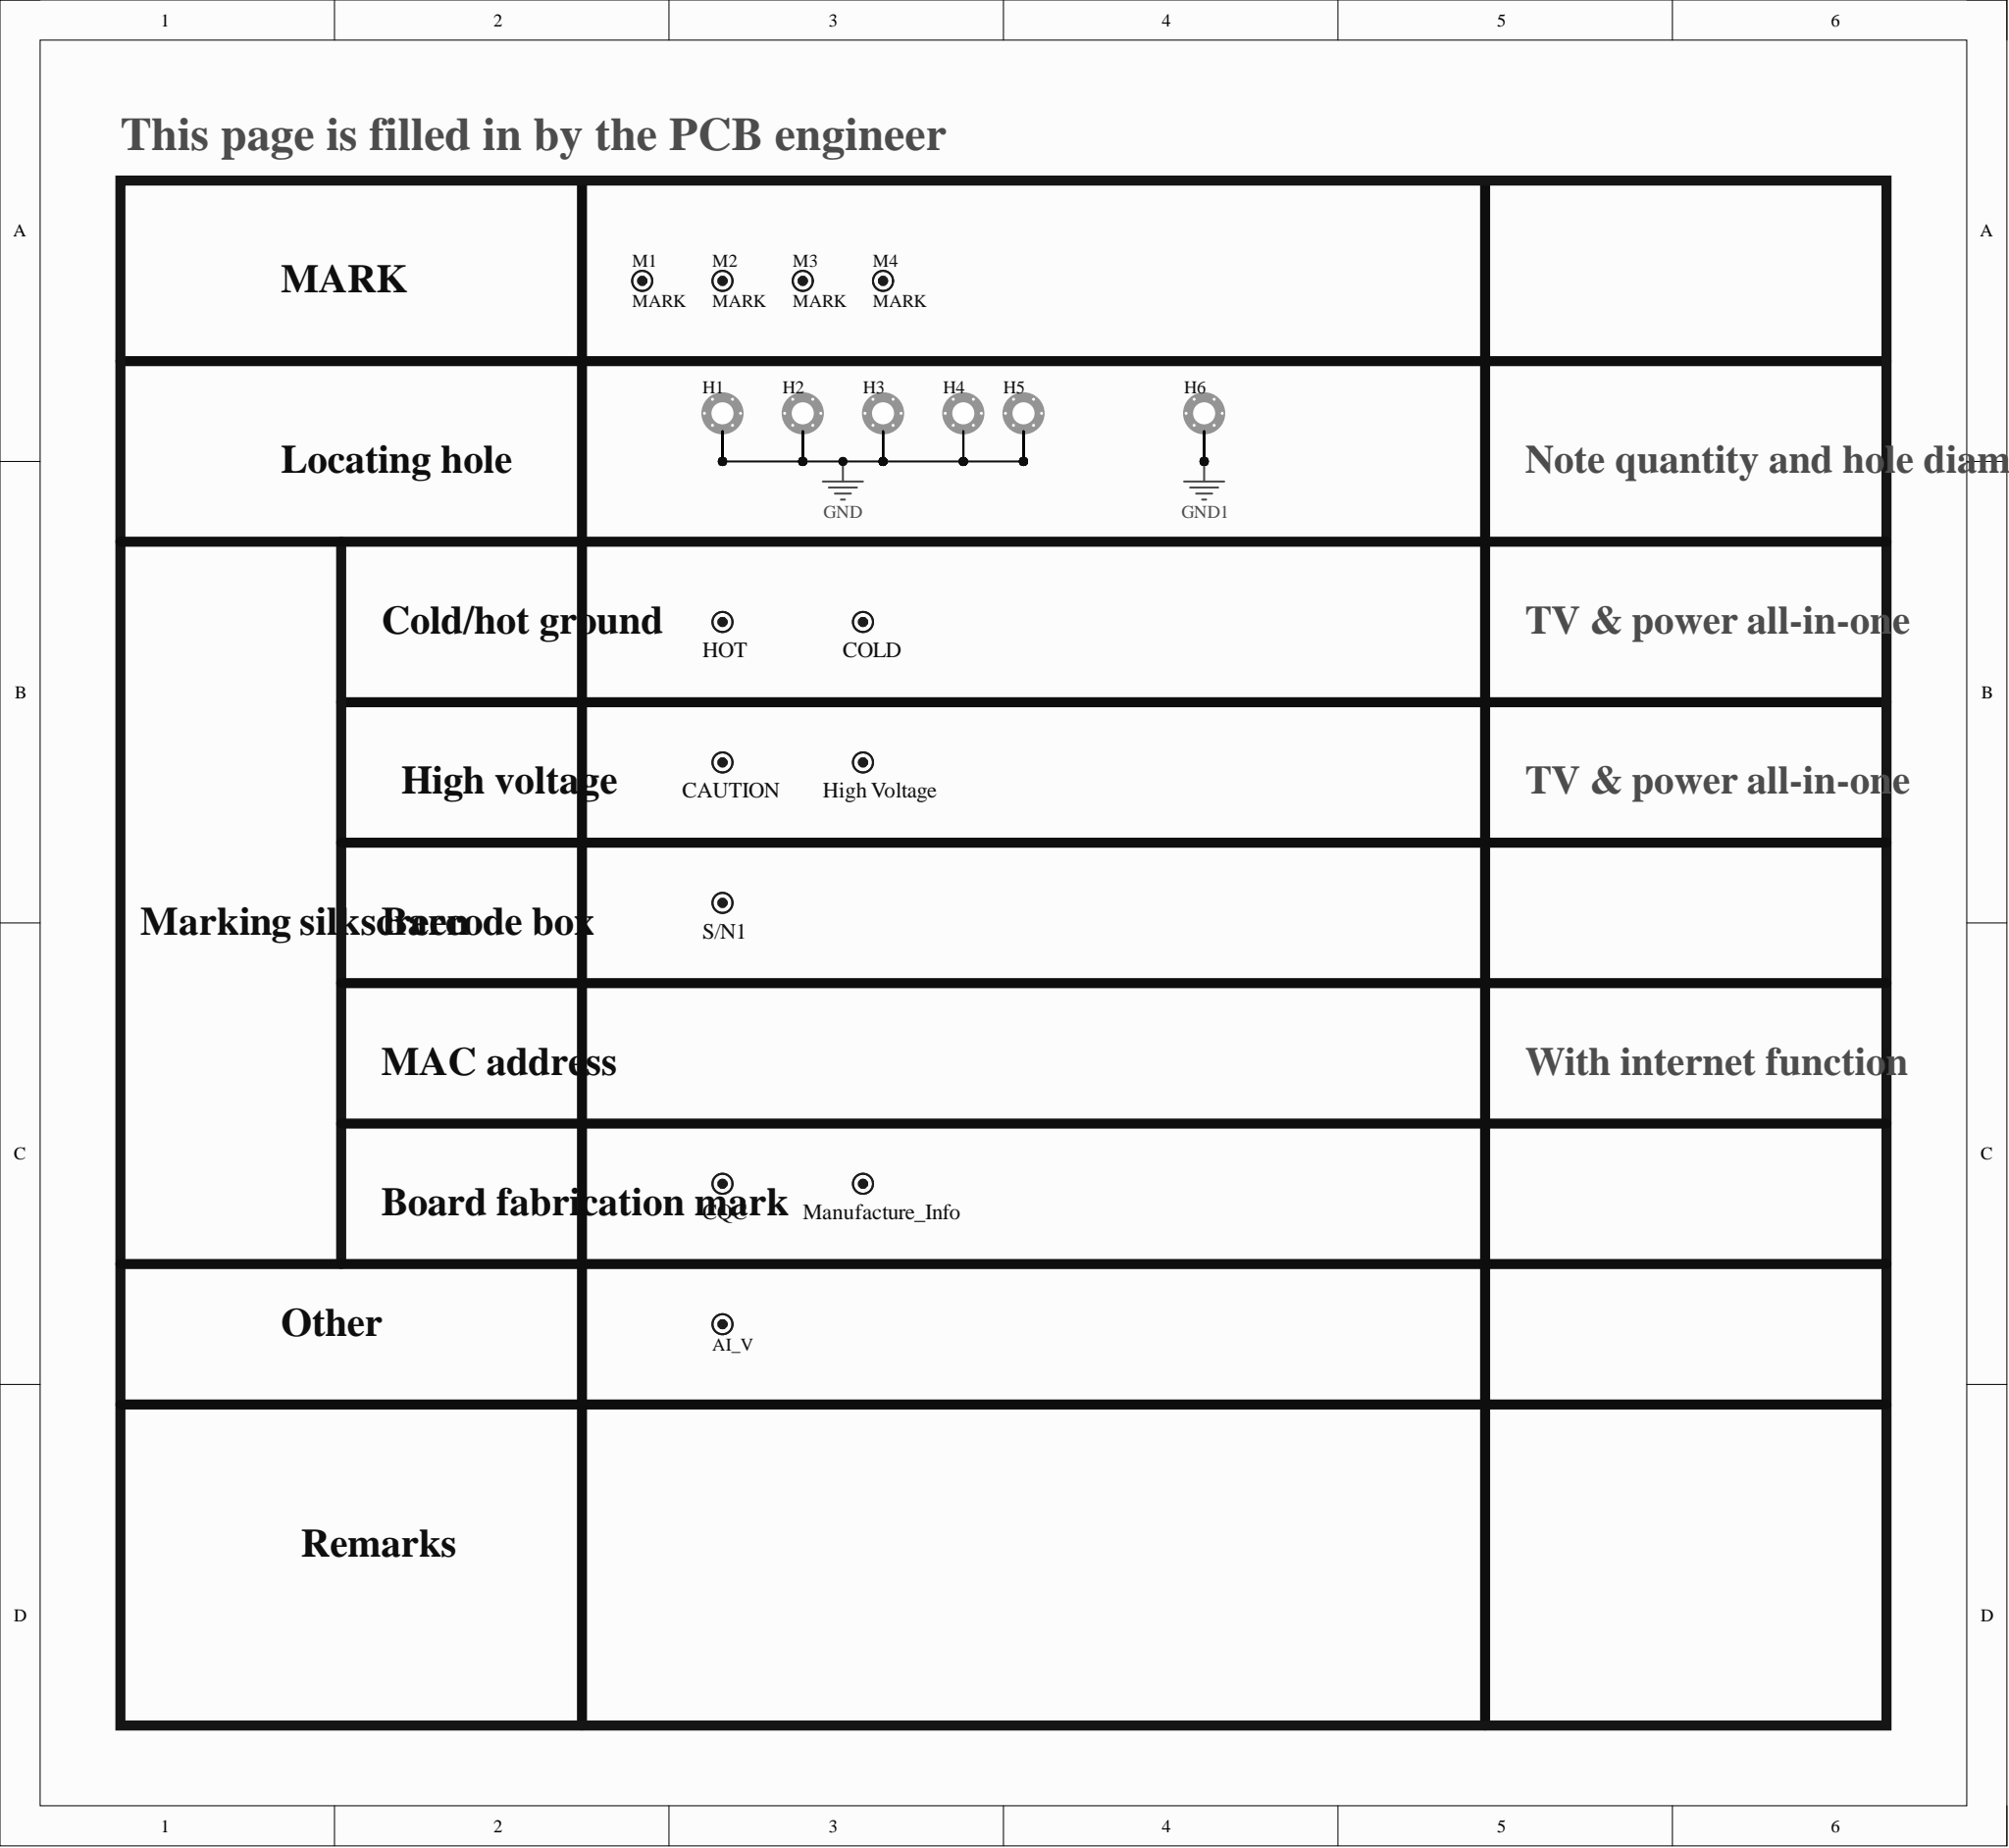Circuit board | Altium Designer | 578 parts | 300 nets | one sheet of the schematic
Parts on this sheet (reference | value | footprint):
AI_V | AI_GRIPPER_V | AI_GRIPPER_V
CAUTION | CAUTION | CAUTION
COLD | COLD | COLD
CQC | CQC | CQC
H1 | Location hole | ASSE4.0C-3
H2 | Location hole | ASSE3.5C-3
H3 | Location hole | ASSE3.5C-3
H4 | Location hole | ASSE5.0C-3
H5 | Location hole | ASSE3.5C-3
H6 | Location hole | ASSE3.5C-3
HOT | HOT | HOT
M1 | MARK | MARK
M2 | MARK | MARK
M3 | MARK | MARK
M4 | MARK | MARK
Manufacture_Info | Manufacture_Info | Manufacture_Info
S/N1 | Barcode | Barcode
Nets of these parts (net: part-pin ...):
GND1: H6-1 H6-2 H6-3 H6-4 H6-5 H6-6
GND: H1-1 H1-2 H1-3 H1-4 H1-5 H1-6 H2-1 H2-2 H2-3 H2-4 H2-5 H2-6 H3-1 H3-2 H3-3 H3-4 H3-5 H3-6 H4-1 H4-2 H4-3 H4-4 H4-5 H4-6 H5-1 H5-2 H5-3 H5-4 H5-5 H5-6